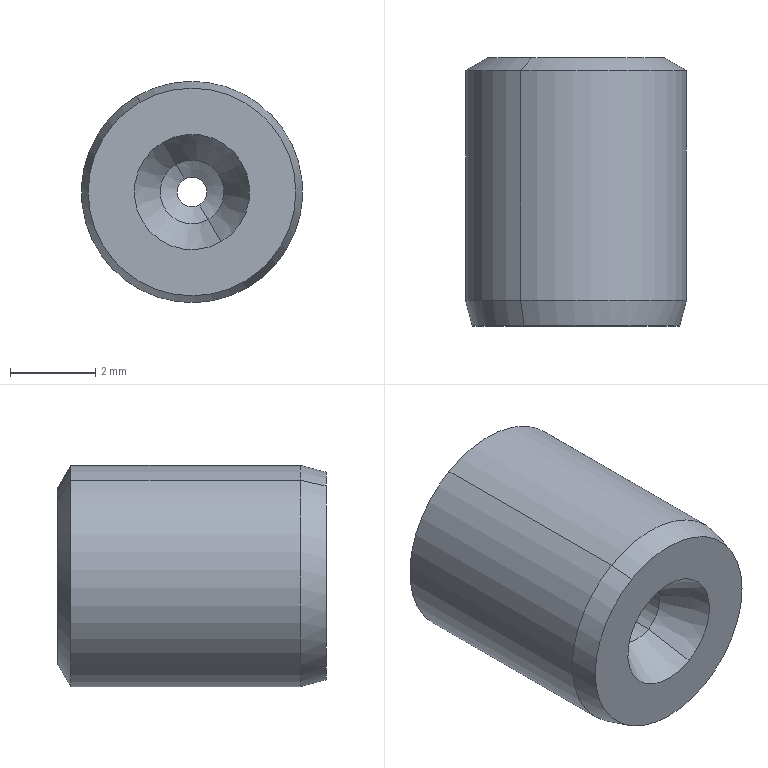Part | SolidWorks | features BaseBody 1 | 1 solid | 18 faces | box 5.2 x 6.3 x 5.2 mm | volume 121.335 mm3 | cone 10 | cylinder 6 | plane 2 | commonest cylinder face diameters 0.7 x2 1.5 x2 5.2 x2
STEP:
#1=CARTESIAN_POINT('',(229.125,175.5,0.6495));
#2=VERTEX_POINT('',#1);
#3=CARTESIAN_POINT('',(229.875,175.5,-0.6495));
#4=VERTEX_POINT('',#3);
#5=CARTESIAN_POINT('',(229.5,175.5,0.));
#6=DIRECTION('',(0.,-1.,0.));
#7=DIRECTION('',(0.5,0.,-0.866));
#8=AXIS2_PLACEMENT_3D('',#5,#6,#7);
#9=CIRCLE('',#8,0.75);
#10=EDGE_CURVE('',#2,#4,#9,.T.);
#11=ORIENTED_EDGE('',*,*,#10,.F.);
#12=CARTESIAN_POINT('',(229.125,172.351,0.6495));
#13=VERTEX_POINT('',#12);
#14=CARTESIAN_POINT('',(229.125,170.118,0.6495));
#15=DIRECTION('',(0.,-1.,0.));
#16=VECTOR('',#15,1000.);
#17=LINE('',#14,#16);
#18=EDGE_CURVE('',#2,#13,#17,.T.);
#19=ORIENTED_EDGE('',*,*,#18,.T.);
#20=CARTESIAN_POINT('',(229.875,172.351,-0.6495));
#21=VERTEX_POINT('',#20);
#22=CARTESIAN_POINT('',(229.5,172.351,0.));
#23=DIRECTION('',(0.,-1.,0.));
#24=DIRECTION('',(0.5,0.,-0.866));
#25=AXIS2_PLACEMENT_3D('',#22,#23,#24);
#26=CIRCLE('',#25,0.75);
#27=EDGE_CURVE('',#13,#21,#26,.T.);
#28=ORIENTED_EDGE('',*,*,#27,.T.);
#29=CARTESIAN_POINT('',(229.875,170.118,-0.6495));
#30=DIRECTION('',(0.,-1.,0.));
#31=VECTOR('',#30,1000.);
#32=LINE('',#29,#31);
#33=EDGE_CURVE('',#4,#21,#32,.T.);
#34=ORIENTED_EDGE('',*,*,#33,.F.);
#35=EDGE_LOOP('',(#11,#19,#28,#34));
#36=FACE_OUTER_BOUND('',#35,.T.);
#37=CARTESIAN_POINT('',(229.5,170.118,0.));
#38=DIRECTION('',(0.,-1.,0.));
#39=DIRECTION('',(0.5,0.,-0.866));
#40=AXIS2_PLACEMENT_3D('',#37,#38,#39);
#41=CYLINDRICAL_SURFACE('',#40,0.75);
#42=ADVANCED_FACE('',(#36),#41,.F.);
#43=CARTESIAN_POINT('',(229.325,175.731,0.3031));
#44=VERTEX_POINT('',#43);
#45=CARTESIAN_POINT('',(229.675,175.731,-0.3031));
#46=VERTEX_POINT('',#45);
#47=CARTESIAN_POINT('',(229.5,175.731,0.));
#48=DIRECTION('',(0.,-1.,0.));
#49=DIRECTION('',(0.5,0.,-0.866));
#50=AXIS2_PLACEMENT_3D('',#47,#48,#49);
#51=CIRCLE('',#50,0.35);
#52=EDGE_CURVE('',#44,#46,#51,.T.);
#53=ORIENTED_EDGE('',*,*,#52,.F.);
#54=CARTESIAN_POINT('',(229.325,175.731,0.3031));
#55=DIRECTION('',(-0.433,-0.5,0.75));
#56=VECTOR('',#55,1000.);
#57=LINE('',#54,#56);
#58=EDGE_CURVE('',#44,#2,#57,.T.);
#59=ORIENTED_EDGE('',*,*,#58,.T.);
#60=ORIENTED_EDGE('',*,*,#10,.T.);
#61=CARTESIAN_POINT('',(229.675,175.731,-0.3031));
#62=DIRECTION('',(0.433,-0.5,-0.75));
#63=VECTOR('',#62,1000.);
#64=LINE('',#61,#63);
#65=EDGE_CURVE('',#46,#4,#64,.T.);
#66=ORIENTED_EDGE('',*,*,#65,.F.);
#67=EDGE_LOOP('',(#53,#59,#60,#66));
#68=FACE_OUTER_BOUND('',#67,.T.);
#69=CARTESIAN_POINT('',(229.5,175.731,0.));
#70=DIRECTION('',(0.,-1.,0.));
#71=DIRECTION('',(0.5,0.,-0.866));
#72=AXIS2_PLACEMENT_3D('',#69,#70,#71);
#73=CONICAL_SURFACE('',#72,0.35,1.047);
#74=ADVANCED_FACE('',(#68),#73,.F.);
#75=CARTESIAN_POINT('',(229.325,177.08,0.3031));
#76=VERTEX_POINT('',#75);
#77=CARTESIAN_POINT('',(229.675,177.08,-0.3031));
#78=VERTEX_POINT('',#77);
#79=CARTESIAN_POINT('',(229.5,177.08,0.));
#80=DIRECTION('',(0.,-1.,0.));
#81=DIRECTION('',(0.5,0.,-0.866));
#82=AXIS2_PLACEMENT_3D('',#79,#80,#81);
#83=CIRCLE('',#82,0.35);
#84=EDGE_CURVE('',#76,#78,#83,.T.);
#85=ORIENTED_EDGE('',*,*,#84,.F.);
#86=CARTESIAN_POINT('',(229.325,170.118,0.3031));
#87=DIRECTION('',(0.,-1.,0.));
#88=VECTOR('',#87,1000.);
#89=LINE('',#86,#88);
#90=EDGE_CURVE('',#76,#44,#89,.T.);
#91=ORIENTED_EDGE('',*,*,#90,.T.);
#92=ORIENTED_EDGE('',*,*,#52,.T.);
#93=CARTESIAN_POINT('',(229.675,170.118,-0.3031));
#94=DIRECTION('',(0.,-1.,0.));
#95=VECTOR('',#94,1000.);
#96=LINE('',#93,#95);
#97=EDGE_CURVE('',#78,#46,#96,.T.);
#98=ORIENTED_EDGE('',*,*,#97,.F.);
#99=EDGE_LOOP('',(#85,#91,#92,#98));
#100=FACE_OUTER_BOUND('',#99,.T.);
#101=CARTESIAN_POINT('',(229.5,170.118,0.));
#102=DIRECTION('',(0.,-1.,0.));
#103=DIRECTION('',(0.5,0.,-0.866));
#104=AXIS2_PLACEMENT_3D('',#101,#102,#103);
#105=CYLINDRICAL_SURFACE('',#104,0.35);
#106=ADVANCED_FACE('',(#100),#105,.F.);
#107=ORIENTED_EDGE('',*,*,#84,.T.);
#108=CARTESIAN_POINT('',(229.825,177.6,-0.5629));
#109=VERTEX_POINT('',#108);
#110=CARTESIAN_POINT('',(229.825,177.6,-0.5629));
#111=DIRECTION('',(0.25,0.866,-0.433));
#112=VECTOR('',#111,1000.);
#113=LINE('',#110,#112);
#114=EDGE_CURVE('',#78,#109,#113,.T.);
#115=ORIENTED_EDGE('',*,*,#114,.T.);
#116=CARTESIAN_POINT('',(229.175,177.6,0.5629));
#117=VERTEX_POINT('',#116);
#118=CARTESIAN_POINT('',(229.5,177.6,0.));
#119=DIRECTION('',(0.,-1.,0.));
#120=DIRECTION('',(0.5,0.,-0.866));
#121=AXIS2_PLACEMENT_3D('',#118,#119,#120);
#122=CIRCLE('',#121,0.65);
#123=EDGE_CURVE('',#117,#109,#122,.T.);
#124=ORIENTED_EDGE('',*,*,#123,.F.);
#125=CARTESIAN_POINT('',(229.175,177.6,0.5629));
#126=DIRECTION('',(-0.25,0.866,0.433));
#127=VECTOR('',#126,1000.);
#128=LINE('',#125,#127);
#129=EDGE_CURVE('',#76,#117,#128,.T.);
#130=ORIENTED_EDGE('',*,*,#129,.F.);
#131=EDGE_LOOP('',(#107,#115,#124,#130));
#132=FACE_OUTER_BOUND('',#131,.T.);
#133=CARTESIAN_POINT('',(229.5,177.6,0.));
#134=DIRECTION('',(0.,1.,0.));
#135=DIRECTION('',(-0.5,0.,0.866));
#136=AXIS2_PLACEMENT_3D('',#133,#134,#135);
#137=CONICAL_SURFACE('',#136,0.65,0.5236);
#138=ADVANCED_FACE('',(#132),#137,.F.);
#139=CARTESIAN_POINT('',(230.54,177.6,-1.802));
#140=VERTEX_POINT('',#139);
#141=CARTESIAN_POINT('',(228.46,177.6,1.802));
#142=VERTEX_POINT('',#141);
#143=CARTESIAN_POINT('',(229.5,177.6,0.));
#144=DIRECTION('',(0.,-1.,0.));
#145=DIRECTION('',(0.5,0.,-0.866));
#146=AXIS2_PLACEMENT_3D('',#143,#144,#145);
#147=CIRCLE('',#146,2.08);
#148=EDGE_CURVE('',#140,#142,#147,.T.);
#149=ORIENTED_EDGE('',*,*,#148,.T.);
#150=CARTESIAN_POINT('',(228.2,177.3,2.252));
#151=VERTEX_POINT('',#150);
#152=CARTESIAN_POINT('',(228.2,177.3,2.252));
#153=DIRECTION('',(-0.433,-0.5,0.75));
#154=VECTOR('',#153,1000.);
#155=LINE('',#152,#154);
#156=EDGE_CURVE('',#142,#151,#155,.T.);
#157=ORIENTED_EDGE('',*,*,#156,.T.);
#158=CARTESIAN_POINT('',(230.8,177.3,-2.252));
#159=VERTEX_POINT('',#158);
#160=CARTESIAN_POINT('',(229.5,177.3,0.));
#161=DIRECTION('',(0.,-1.,0.));
#162=DIRECTION('',(0.5,0.,-0.866));
#163=AXIS2_PLACEMENT_3D('',#160,#161,#162);
#164=CIRCLE('',#163,2.6);
#165=EDGE_CURVE('',#159,#151,#164,.T.);
#166=ORIENTED_EDGE('',*,*,#165,.F.);
#167=CARTESIAN_POINT('',(230.8,177.3,-2.252));
#168=DIRECTION('',(0.433,-0.5,-0.75));
#169=VECTOR('',#168,1000.);
#170=LINE('',#167,#169);
#171=EDGE_CURVE('',#140,#159,#170,.T.);
#172=ORIENTED_EDGE('',*,*,#171,.F.);
#173=EDGE_LOOP('',(#149,#157,#166,#172));
#174=FACE_OUTER_BOUND('',#173,.T.);
#175=CARTESIAN_POINT('',(229.5,177.3,0.));
#176=DIRECTION('',(0.,-1.,0.));
#177=DIRECTION('',(0.5,0.,-0.866));
#178=AXIS2_PLACEMENT_3D('',#175,#176,#177);
#179=CONICAL_SURFACE('',#178,2.6,1.047);
#180=ADVANCED_FACE('',(#174),#179,.T.);
#181=ORIENTED_EDGE('',*,*,#165,.T.);
#182=CARTESIAN_POINT('',(228.2,171.9,2.252));
#183=VERTEX_POINT('',#182);
#184=CARTESIAN_POINT('',(228.2,170.118,2.252));
#185=DIRECTION('',(0.,-1.,0.));
#186=VECTOR('',#185,1000.);
#187=LINE('',#184,#186);
#188=EDGE_CURVE('',#151,#183,#187,.T.);
#189=ORIENTED_EDGE('',*,*,#188,.T.);
#190=CARTESIAN_POINT('',(230.8,171.9,-2.252));
#191=VERTEX_POINT('',#190);
#192=CARTESIAN_POINT('',(229.5,171.9,0.));
#193=DIRECTION('',(0.,-1.,0.));
#194=DIRECTION('',(0.5,0.,-0.866));
#195=AXIS2_PLACEMENT_3D('',#192,#193,#194);
#196=CIRCLE('',#195,2.6);
#197=EDGE_CURVE('',#191,#183,#196,.T.);
#198=ORIENTED_EDGE('',*,*,#197,.F.);
#199=CARTESIAN_POINT('',(230.8,170.118,-2.252));
#200=DIRECTION('',(0.,-1.,0.));
#201=VECTOR('',#200,1000.);
#202=LINE('',#199,#201);
#203=EDGE_CURVE('',#159,#191,#202,.T.);
#204=ORIENTED_EDGE('',*,*,#203,.F.);
#205=EDGE_LOOP('',(#181,#189,#198,#204));
#206=FACE_OUTER_BOUND('',#205,.T.);
#207=CARTESIAN_POINT('',(229.5,170.118,0.));
#208=DIRECTION('',(0.,-1.,0.));
#209=DIRECTION('',(0.5,0.,-0.866));
#210=AXIS2_PLACEMENT_3D('',#207,#208,#209);
#211=CYLINDRICAL_SURFACE('',#210,2.6);
#212=ADVANCED_FACE('',(#206),#211,.T.);
#213=CARTESIAN_POINT('',(230.72,171.3,-2.112));
#214=VERTEX_POINT('',#213);
#215=CARTESIAN_POINT('',(228.28,171.3,2.112));
#216=VERTEX_POINT('',#215);
#217=CARTESIAN_POINT('',(229.5,171.3,0.));
#218=DIRECTION('',(0.,-1.,0.));
#219=DIRECTION('',(0.5,0.,-0.866));
#220=AXIS2_PLACEMENT_3D('',#217,#218,#219);
#221=CIRCLE('',#220,2.439);
#222=EDGE_CURVE('',#214,#216,#221,.T.);
#223=ORIENTED_EDGE('',*,*,#222,.F.);
#224=CARTESIAN_POINT('',(230.72,171.3,-2.112));
#225=DIRECTION('',(0.1294,0.9659,-0.2241));
#226=VECTOR('',#225,1000.);
#227=LINE('',#224,#226);
#228=EDGE_CURVE('',#214,#191,#227,.T.);
#229=ORIENTED_EDGE('',*,*,#228,.T.);
#230=ORIENTED_EDGE('',*,*,#197,.T.);
#231=CARTESIAN_POINT('',(228.28,171.3,2.112));
#232=DIRECTION('',(-0.1294,0.9659,0.2241));
#233=VECTOR('',#232,1000.);
#234=LINE('',#231,#233);
#235=EDGE_CURVE('',#216,#183,#234,.T.);
#236=ORIENTED_EDGE('',*,*,#235,.F.);
#237=EDGE_LOOP('',(#223,#229,#230,#236));
#238=FACE_OUTER_BOUND('',#237,.T.);
#239=CARTESIAN_POINT('',(229.5,171.3,0.));
#240=DIRECTION('',(0.,1.,0.));
#241=DIRECTION('',(-0.5,0.,0.866));
#242=AXIS2_PLACEMENT_3D('',#239,#240,#241);
#243=CONICAL_SURFACE('',#242,2.439,0.2618);
#244=ADVANCED_FACE('',(#238),#243,.T.);
#245=ORIENTED_EDGE('',*,*,#27,.F.);
#246=CARTESIAN_POINT('',(228.822,171.3,1.175));
#247=VERTEX_POINT('',#246);
#248=CARTESIAN_POINT('',(229.125,172.351,0.6495));
#249=DIRECTION('',(-0.25,-0.866,0.433));
#250=VECTOR('',#249,1000.);
#251=LINE('',#248,#250);
#252=EDGE_CURVE('',#13,#247,#251,.T.);
#253=ORIENTED_EDGE('',*,*,#252,.T.);
#254=CARTESIAN_POINT('',(230.178,171.3,-1.175));
#255=VERTEX_POINT('',#254);
#256=CARTESIAN_POINT('',(229.5,171.3,0.));
#257=DIRECTION('',(0.,-1.,0.));
#258=DIRECTION('',(0.5,0.,-0.866));
#259=AXIS2_PLACEMENT_3D('',#256,#257,#258);
#260=CIRCLE('',#259,1.357);
#261=EDGE_CURVE('',#247,#255,#260,.T.);
#262=ORIENTED_EDGE('',*,*,#261,.T.);
#263=CARTESIAN_POINT('',(229.875,172.351,-0.6495));
#264=DIRECTION('',(0.25,-0.866,-0.433));
#265=VECTOR('',#264,1000.);
#266=LINE('',#263,#265);
#267=EDGE_CURVE('',#21,#255,#266,.T.);
#268=ORIENTED_EDGE('',*,*,#267,.F.);
#269=EDGE_LOOP('',(#245,#253,#262,#268));
#270=FACE_OUTER_BOUND('',#269,.T.);
#271=CARTESIAN_POINT('',(229.5,172.351,0.));
#272=DIRECTION('',(0.,-1.,0.));
#273=DIRECTION('',(0.5,0.,-0.866));
#274=AXIS2_PLACEMENT_3D('',#271,#272,#273);
#275=CONICAL_SURFACE('',#274,0.75,0.5236);
#276=ADVANCED_FACE('',(#270),#275,.F.);
#277=ORIENTED_EDGE('',*,*,#252,.F.);
#278=CARTESIAN_POINT('',(229.5,172.351,0.));
#279=DIRECTION('',(0.,-1.,0.));
#280=DIRECTION('',(0.5,0.,-0.866));
#281=AXIS2_PLACEMENT_3D('',#278,#279,#280);
#282=CIRCLE('',#281,0.75);
#283=EDGE_CURVE('',#21,#13,#282,.T.);
#284=ORIENTED_EDGE('',*,*,#283,.F.);
#285=ORIENTED_EDGE('',*,*,#267,.T.);
#286=CARTESIAN_POINT('',(229.5,171.3,0.));
#287=DIRECTION('',(0.,-1.,0.));
#288=DIRECTION('',(0.5,0.,-0.866));
#289=AXIS2_PLACEMENT_3D('',#286,#287,#288);
#290=CIRCLE('',#289,1.357);
#291=EDGE_CURVE('',#255,#247,#290,.T.);
#292=ORIENTED_EDGE('',*,*,#291,.T.);
#293=EDGE_LOOP('',(#277,#284,#285,#292));
#294=FACE_OUTER_BOUND('',#293,.T.);
#295=CARTESIAN_POINT('',(229.5,172.351,0.));
#296=DIRECTION('',(0.,-1.,0.));
#297=DIRECTION('',(0.5,0.,-0.866));
#298=AXIS2_PLACEMENT_3D('',#295,#296,#297);
#299=CONICAL_SURFACE('',#298,0.75,0.5236);
#300=ADVANCED_FACE('',(#294),#299,.F.);
#301=CARTESIAN_POINT('',(229.5,171.3,0.));
#302=DIRECTION('',(0.,-1.,0.));
#303=DIRECTION('',(0.5,0.,-0.866));
#304=AXIS2_PLACEMENT_3D('',#301,#302,#303);
#305=CIRCLE('',#304,2.439);
#306=EDGE_CURVE('',#216,#214,#305,.T.);
#307=ORIENTED_EDGE('',*,*,#306,.T.);
#308=ORIENTED_EDGE('',*,*,#222,.T.);
#309=EDGE_LOOP('',(#307,#308));
#310=FACE_OUTER_BOUND('',#309,.T.);
#311=ORIENTED_EDGE('',*,*,#291,.F.);
#312=ORIENTED_EDGE('',*,*,#261,.F.);
#313=EDGE_LOOP('',(#311,#312));
#314=FACE_BOUND('',#313,.T.);
#315=CARTESIAN_POINT('',(230.675,171.3,0.6784));
#316=DIRECTION('',(0.,-1.,0.));
#317=DIRECTION('',(0.5,0.,-0.866));
#318=AXIS2_PLACEMENT_3D('',#315,#316,#317);
#319=PLANE('',#318);
#320=ADVANCED_FACE('',(#310,#314),#319,.T.);
#321=ORIENTED_EDGE('',*,*,#228,.F.);
#322=ORIENTED_EDGE('',*,*,#306,.F.);
#323=ORIENTED_EDGE('',*,*,#235,.T.);
#324=CARTESIAN_POINT('',(229.5,171.9,0.));
#325=DIRECTION('',(0.,-1.,0.));
#326=DIRECTION('',(0.5,0.,-0.866));
#327=AXIS2_PLACEMENT_3D('',#324,#325,#326);
#328=CIRCLE('',#327,2.6);
#329=EDGE_CURVE('',#183,#191,#328,.T.);
#330=ORIENTED_EDGE('',*,*,#329,.T.);
#331=EDGE_LOOP('',(#321,#322,#323,#330));
#332=FACE_OUTER_BOUND('',#331,.T.);
#333=CARTESIAN_POINT('',(229.5,171.3,0.));
#334=DIRECTION('',(0.,1.,0.));
#335=DIRECTION('',(-0.5,0.,0.866));
#336=AXIS2_PLACEMENT_3D('',#333,#334,#335);
#337=CONICAL_SURFACE('',#336,2.439,0.2618);
#338=ADVANCED_FACE('',(#332),#337,.T.);
#339=ORIENTED_EDGE('',*,*,#188,.F.);
#340=CARTESIAN_POINT('',(229.5,177.3,0.));
#341=DIRECTION('',(0.,-1.,0.));
#342=DIRECTION('',(0.5,0.,-0.866));
#343=AXIS2_PLACEMENT_3D('',#340,#341,#342);
#344=CIRCLE('',#343,2.6);
#345=EDGE_CURVE('',#151,#159,#344,.T.);
#346=ORIENTED_EDGE('',*,*,#345,.T.);
#347=ORIENTED_EDGE('',*,*,#203,.T.);
#348=ORIENTED_EDGE('',*,*,#329,.F.);
#349=EDGE_LOOP('',(#339,#346,#347,#348));
#350=FACE_OUTER_BOUND('',#349,.T.);
#351=CARTESIAN_POINT('',(229.5,170.118,0.));
#352=DIRECTION('',(0.,-1.,0.));
#353=DIRECTION('',(0.5,0.,-0.866));
#354=AXIS2_PLACEMENT_3D('',#351,#352,#353);
#355=CYLINDRICAL_SURFACE('',#354,2.6);
#356=ADVANCED_FACE('',(#350),#355,.T.);
#357=ORIENTED_EDGE('',*,*,#156,.F.);
#358=CARTESIAN_POINT('',(229.5,177.6,0.));
#359=DIRECTION('',(0.,-1.,0.));
#360=DIRECTION('',(0.5,0.,-0.866));
#361=AXIS2_PLACEMENT_3D('',#358,#359,#360);
#362=CIRCLE('',#361,2.08);
#363=EDGE_CURVE('',#142,#140,#362,.T.);
#364=ORIENTED_EDGE('',*,*,#363,.T.);
#365=ORIENTED_EDGE('',*,*,#171,.T.);
#366=ORIENTED_EDGE('',*,*,#345,.F.);
#367=EDGE_LOOP('',(#357,#364,#365,#366));
#368=FACE_OUTER_BOUND('',#367,.T.);
#369=CARTESIAN_POINT('',(229.5,177.3,0.));
#370=DIRECTION('',(0.,-1.,0.));
#371=DIRECTION('',(0.5,0.,-0.866));
#372=AXIS2_PLACEMENT_3D('',#369,#370,#371);
#373=CONICAL_SURFACE('',#372,2.6,1.047);
#374=ADVANCED_FACE('',(#368),#373,.T.);
#375=ORIENTED_EDGE('',*,*,#123,.T.);
#376=CARTESIAN_POINT('',(229.5,177.6,0.));
#377=DIRECTION('',(0.,-1.,0.));
#378=DIRECTION('',(0.5,0.,-0.866));
#379=AXIS2_PLACEMENT_3D('',#376,#377,#378);
#380=CIRCLE('',#379,0.65);
#381=EDGE_CURVE('',#109,#117,#380,.T.);
#382=ORIENTED_EDGE('',*,*,#381,.T.);
#383=EDGE_LOOP('',(#375,#382));
#384=FACE_BOUND('',#383,.T.);
#385=ORIENTED_EDGE('',*,*,#148,.F.);
#386=ORIENTED_EDGE('',*,*,#363,.F.);
#387=EDGE_LOOP('',(#385,#386));
#388=FACE_OUTER_BOUND('',#387,.T.);
#389=CARTESIAN_POINT('',(231.302,177.6,1.04));
#390=DIRECTION('',(0.,1.,0.));
#391=DIRECTION('',(-0.5,0.,0.866));
#392=AXIS2_PLACEMENT_3D('',#389,#390,#391);
#393=PLANE('',#392);
#394=ADVANCED_FACE('',(#384,#388),#393,.T.);
#395=ORIENTED_EDGE('',*,*,#114,.F.);
#396=CARTESIAN_POINT('',(229.5,177.08,0.));
#397=DIRECTION('',(0.,-1.,0.));
#398=DIRECTION('',(0.5,0.,-0.866));
#399=AXIS2_PLACEMENT_3D('',#396,#397,#398);
#400=CIRCLE('',#399,0.35);
#401=EDGE_CURVE('',#78,#76,#400,.T.);
#402=ORIENTED_EDGE('',*,*,#401,.T.);
#403=ORIENTED_EDGE('',*,*,#129,.T.);
#404=ORIENTED_EDGE('',*,*,#381,.F.);
#405=EDGE_LOOP('',(#395,#402,#403,#404));
#406=FACE_OUTER_BOUND('',#405,.T.);
#407=CARTESIAN_POINT('',(229.5,177.6,0.));
#408=DIRECTION('',(0.,1.,0.));
#409=DIRECTION('',(-0.5,0.,0.866));
#410=AXIS2_PLACEMENT_3D('',#407,#408,#409);
#411=CONICAL_SURFACE('',#410,0.65,0.5236);
#412=ADVANCED_FACE('',(#406),#411,.F.);
#413=ORIENTED_EDGE('',*,*,#90,.F.);
#414=ORIENTED_EDGE('',*,*,#401,.F.);
#415=ORIENTED_EDGE('',*,*,#97,.T.);
#416=CARTESIAN_POINT('',(229.5,175.731,0.));
#417=DIRECTION('',(0.,-1.,0.));
#418=DIRECTION('',(0.5,0.,-0.866));
#419=AXIS2_PLACEMENT_3D('',#416,#417,#418);
#420=CIRCLE('',#419,0.35);
#421=EDGE_CURVE('',#46,#44,#420,.T.);
#422=ORIENTED_EDGE('',*,*,#421,.T.);
#423=EDGE_LOOP('',(#413,#414,#415,#422));
#424=FACE_OUTER_BOUND('',#423,.T.);
#425=CARTESIAN_POINT('',(229.5,170.118,0.));
#426=DIRECTION('',(0.,-1.,0.));
#427=DIRECTION('',(0.5,0.,-0.866));
#428=AXIS2_PLACEMENT_3D('',#425,#426,#427);
#429=CYLINDRICAL_SURFACE('',#428,0.35);
#430=ADVANCED_FACE('',(#424),#429,.F.);
#431=ORIENTED_EDGE('',*,*,#58,.F.);
#432=ORIENTED_EDGE('',*,*,#421,.F.);
#433=ORIENTED_EDGE('',*,*,#65,.T.);
#434=CARTESIAN_POINT('',(229.5,175.5,0.));
#435=DIRECTION('',(0.,-1.,0.));
#436=DIRECTION('',(0.5,0.,-0.866));
#437=AXIS2_PLACEMENT_3D('',#434,#435,#436);
#438=CIRCLE('',#437,0.75);
#439=EDGE_CURVE('',#4,#2,#438,.T.);
#440=ORIENTED_EDGE('',*,*,#439,.T.);
#441=EDGE_LOOP('',(#431,#432,#433,#440));
#442=FACE_OUTER_BOUND('',#441,.T.);
#443=CARTESIAN_POINT('',(229.5,175.731,0.));
#444=DIRECTION('',(0.,-1.,0.));
#445=DIRECTION('',(0.5,0.,-0.866));
#446=AXIS2_PLACEMENT_3D('',#443,#444,#445);
#447=CONICAL_SURFACE('',#446,0.35,1.047);
#448=ADVANCED_FACE('',(#442),#447,.F.);
#449=ORIENTED_EDGE('',*,*,#18,.F.);
#450=ORIENTED_EDGE('',*,*,#439,.F.);
#451=ORIENTED_EDGE('',*,*,#33,.T.);
#452=ORIENTED_EDGE('',*,*,#283,.T.);
#453=EDGE_LOOP('',(#449,#450,#451,#452));
#454=FACE_OUTER_BOUND('',#453,.T.);
#455=CARTESIAN_POINT('',(229.5,170.118,0.));
#456=DIRECTION('',(0.,-1.,0.));
#457=DIRECTION('',(0.5,0.,-0.866));
#458=AXIS2_PLACEMENT_3D('',#455,#456,#457);
#459=CYLINDRICAL_SURFACE('',#458,0.75);
#460=ADVANCED_FACE('',(#454),#459,.F.);
#461=CLOSED_SHELL('',(#42,#74,#106,#138,#180,#212,#244,#276,#300,#320,#338,#356,#374,#394,#412,#430,#448,#460));
#462=MANIFOLD_SOLID_BREP('',#461);
#463=CARTESIAN_POINT('',(0.,0.,0.));
#464=DIRECTION('',(0.,0.,1.));
#465=DIRECTION('',(1.,0.,0.));
#466=AXIS2_PLACEMENT_3D('',#463,#464,#465);
#467=(LENGTH_UNIT()NAMED_UNIT(*)SI_UNIT(.MILLI.,.METRE.));
#468=UNCERTAINTY_MEASURE_WITH_UNIT(LENGTH_MEASURE(0.00001),#467,'','');
#469=(NAMED_UNIT(*)PLANE_ANGLE_UNIT()SI_UNIT($,.RADIAN.));
#470=(NAMED_UNIT(*)SI_UNIT($,.STERADIAN.)SOLID_ANGLE_UNIT());
#471=(GEOMETRIC_REPRESENTATION_CONTEXT(3)GLOBAL_UNCERTAINTY_ASSIGNED_CONTEXT((#468))GLOBAL_UNIT_ASSIGNED_CONTEXT((#467,#469,#470))REPRESENTATION_CONTEXT('',''));
#472=ADVANCED_BREP_SHAPE_REPRESENTATION('',(#462,#466),#471);